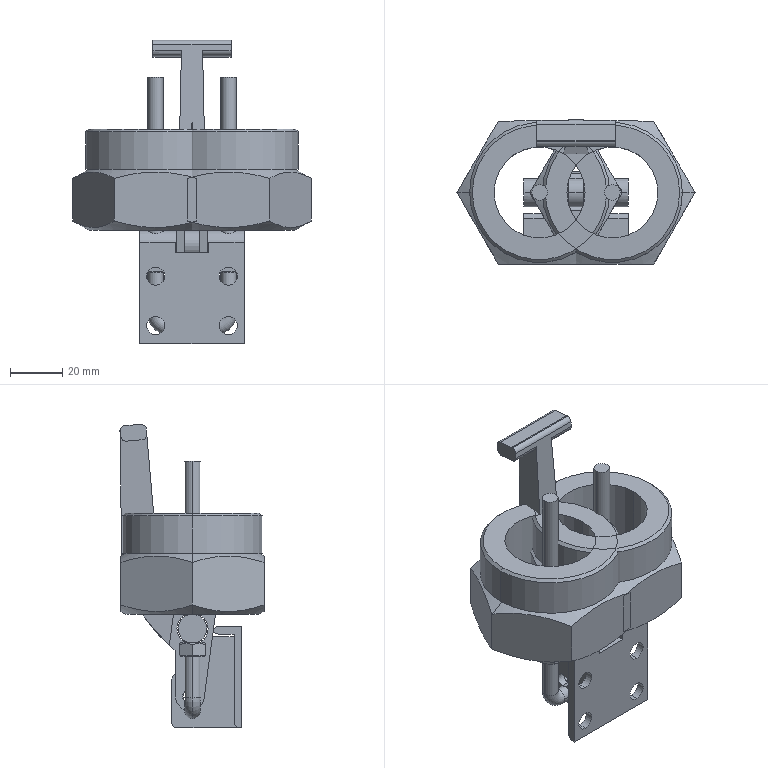Part | SolidWorks | 8 solids | 179 faces | box 91.509 x 55.367 x 116.67 mm | volume 146833 mm3 | plane 78 | cylinder 64 | cone 32 | torus 4 | spline 1 | commonest cylinder face diameters 4 x16 7 x12 6 x6 4.917 x4 5.55 x4 11 x4